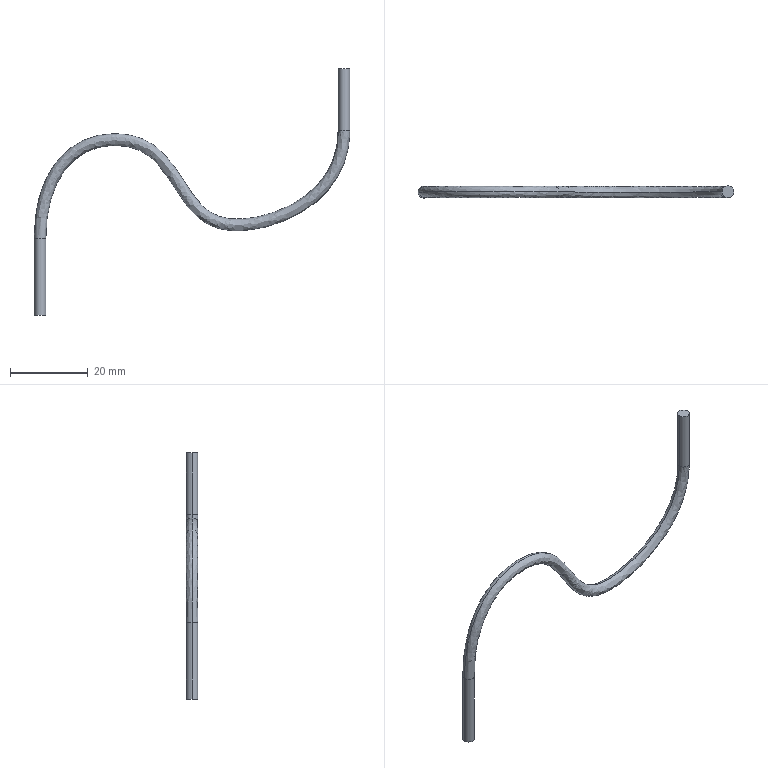Part | SolidWorks | features Sweep 1 | 1 solid | 8 faces | box 81 x 3 x 63.219 mm | volume 1077 mm3 | cylinder 4 | spline 2 | plane 2 | commonest cylinder face diameters 3 x4
STEP:
#1=CARTESIAN_POINT('',(1.5,0.,19.693));
#2=VERTEX_POINT('',#1);
#3=CARTESIAN_POINT('',(-1.5,0.,19.693));
#4=VERTEX_POINT('',#3);
#5=CARTESIAN_POINT('',(0.,0.,19.693));
#6=DIRECTION('',(0.,0.,1.));
#7=DIRECTION('',(1.,0.,0.));
#8=AXIS2_PLACEMENT_3D('',#5,#6,#7);
#9=CIRCLE('',#8,1.5);
#10=EDGE_CURVE('',#2,#4,#9,.T.);
#11=ORIENTED_EDGE('',*,*,#10,.T.);
#12=CARTESIAN_POINT('',(76.5,0.,47.415));
#13=VERTEX_POINT('',#12);
#14=CARTESIAN_POINT('',(-1.5,0.,19.693));
#15=CARTESIAN_POINT('',(-1.5,0.,21.619));
#16=CARTESIAN_POINT('',(-1.286,0.,25.174));
#17=CARTESIAN_POINT('',(-0.3655,0.,30.046));
#18=CARTESIAN_POINT('',(1.116,0.,34.324));
#19=CARTESIAN_POINT('',(3.12,0.,38.02));
#20=CARTESIAN_POINT('',(5.605,0.,41.101));
#21=CARTESIAN_POINT('',(8.521,0.,43.535));
#22=CARTESIAN_POINT('',(11.671,0.,45.218));
#23=CARTESIAN_POINT('',(14.048,0.,45.947));
#24=CARTESIAN_POINT('',(16.493,0.,46.438));
#25=CARTESIAN_POINT('',(19.145,0.,46.678));
#26=CARTESIAN_POINT('',(21.729,0.,46.471));
#27=CARTESIAN_POINT('',(23.985,0.,46.05));
#28=CARTESIAN_POINT('',(26.086,0.,45.432));
#29=CARTESIAN_POINT('',(29.579,0.,43.628));
#30=CARTESIAN_POINT('',(33.041,0.,40.317));
#31=CARTESIAN_POINT('',(36.143,0.,35.723));
#32=CARTESIAN_POINT('',(38.926,0.,31.213));
#33=CARTESIAN_POINT('',(41.349,0.,28.227));
#34=CARTESIAN_POINT('',(43.255,0.,26.716));
#35=CARTESIAN_POINT('',(44.276,0.,26.089));
#36=CARTESIAN_POINT('',(45.357,0.,25.543));
#37=CARTESIAN_POINT('',(46.813,0.,25.02));
#38=CARTESIAN_POINT('',(48.557,0.,24.717));
#39=CARTESIAN_POINT('',(50.199,0.,24.626));
#40=CARTESIAN_POINT('',(52.606,0.,24.658));
#41=CARTESIAN_POINT('',(56.696,0.,25.233));
#42=CARTESIAN_POINT('',(62.394,0.,27.105));
#43=CARTESIAN_POINT('',(67.129,0.,29.763));
#44=CARTESIAN_POINT('',(70.632,0.,32.74));
#45=CARTESIAN_POINT('',(73.067,0.,35.628));
#46=CARTESIAN_POINT('',(74.957,0.,39.));
#47=CARTESIAN_POINT('',(76.193,0.,42.844));
#48=CARTESIAN_POINT('',(76.5,0.,45.884));
#49=CARTESIAN_POINT('',(76.5,0.,47.415));
#50=B_SPLINE_CURVE_WITH_KNOTS('',3,(#14,#15,#16,#17,#18,#19,#20,#21,#22,#23,#24,#25,#26,#27,#28,#29,#30,#31,#32,#33,#34,#35,#36,#37,#38,#39,#40,#41,#42,#43,#44,#45,#46,#47,#48,#49),.UNSPECIFIED.,.F.,.F.,(4,1,1,1,1,1,1,1,1,1,1,1,1,1,1,1,1,1,1,1,1,1,1,1,1,1,1,1,1,1,1,1,1,4),(0.,0.03125,0.0625,0.09375,0.125,0.1562,0.1875,0.2188,0.2463,0.25,0.2812,0.3125,0.317,0.3437,0.375,0.4375,0.5,0.5625,0.625,0.65,0.6638,0.675,0.7,0.725,0.7364,0.75,0.7917,0.8333,0.875,0.9,0.925,0.95,0.975,1.),.UNSPECIFIED.);
#51=EDGE_CURVE('',#4,#13,#50,.T.);
#52=ORIENTED_EDGE('',*,*,#51,.T.);
#53=CARTESIAN_POINT('',(79.5,0.,47.415));
#54=VERTEX_POINT('',#53);
#55=CARTESIAN_POINT('',(78.,0.,47.415));
#56=DIRECTION('',(0.,0.,1.));
#57=DIRECTION('',(1.,0.,0.));
#58=AXIS2_PLACEMENT_3D('',#55,#56,#57);
#59=CIRCLE('',#58,1.5);
#60=EDGE_CURVE('',#54,#13,#59,.T.);
#61=ORIENTED_EDGE('',*,*,#60,.F.);
#62=CARTESIAN_POINT('',(1.5,0.,19.693));
#63=CARTESIAN_POINT('',(1.5,0.,21.529));
#64=CARTESIAN_POINT('',(1.701,0.,24.81));
#65=CARTESIAN_POINT('',(2.548,0.,29.292));
#66=CARTESIAN_POINT('',(3.881,0.,33.125));
#67=CARTESIAN_POINT('',(5.64,0.,36.362));
#68=CARTESIAN_POINT('',(7.767,0.,38.993));
#69=CARTESIAN_POINT('',(10.214,0.,41.032));
#70=CARTESIAN_POINT('',(12.837,0.,42.433));
#71=CARTESIAN_POINT('',(14.816,0.,43.042));
#72=CARTESIAN_POINT('',(16.882,0.,43.456));
#73=CARTESIAN_POINT('',(19.163,0.,43.665));
#74=CARTESIAN_POINT('',(21.382,0.,43.483));
#75=CARTESIAN_POINT('',(23.262,0.,43.134));
#76=CARTESIAN_POINT('',(24.963,0.,42.63));
#77=CARTESIAN_POINT('',(27.763,0.,41.186));
#78=CARTESIAN_POINT('',(30.672,0.,38.439));
#79=CARTESIAN_POINT('',(33.584,0.,34.163));
#80=CARTESIAN_POINT('',(36.417,0.,29.558));
#81=CARTESIAN_POINT('',(39.152,0.,26.143));
#82=CARTESIAN_POINT('',(41.51,0.,24.266));
#83=CARTESIAN_POINT('',(42.806,0.,23.47));
#84=CARTESIAN_POINT('',(44.192,0.,22.769));
#85=CARTESIAN_POINT('',(46.066,0.,22.098));
#86=CARTESIAN_POINT('',(48.215,0.,21.73));
#87=CARTESIAN_POINT('',(50.146,0.,21.624));
#88=CARTESIAN_POINT('',(52.902,0.,21.663));
#89=CARTESIAN_POINT('',(57.393,0.,22.301));
#90=CARTESIAN_POINT('',(63.599,0.,24.338));
#91=CARTESIAN_POINT('',(68.819,0.,27.261));
#92=CARTESIAN_POINT('',(72.76,0.,30.605));
#93=CARTESIAN_POINT('',(75.544,0.,33.901));
#94=CARTESIAN_POINT('',(77.729,0.,37.803));
#95=CARTESIAN_POINT('',(79.155,0.,42.223));
#96=CARTESIAN_POINT('',(79.5,0.,45.734));
#97=CARTESIAN_POINT('',(79.5,0.,47.415));
#98=B_SPLINE_CURVE_WITH_KNOTS('',3,(#62,#63,#64,#65,#66,#67,#68,#69,#70,#71,#72,#73,#74,#75,#76,#77,#78,#79,#80,#81,#82,#83,#84,#85,#86,#87,#88,#89,#90,#91,#92,#93,#94,#95,#96,#97),.UNSPECIFIED.,.F.,.F.,(4,1,1,1,1,1,1,1,1,1,1,1,1,1,1,1,1,1,1,1,1,1,1,1,1,1,1,1,1,1,1,1,1,4),(0.,0.03125,0.0625,0.09375,0.125,0.1562,0.1875,0.2188,0.2463,0.25,0.2812,0.3125,0.317,0.3437,0.375,0.4375,0.5,0.5625,0.625,0.65,0.6638,0.675,0.7,0.725,0.7364,0.75,0.7917,0.8333,0.875,0.9,0.925,0.95,0.975,1.),.UNSPECIFIED.);
#99=EDGE_CURVE('',#2,#54,#98,.T.);
#100=ORIENTED_EDGE('',*,*,#99,.F.);
#101=EDGE_LOOP('',(#11,#52,#61,#100));
#102=FACE_OUTER_BOUND('',#101,.T.);
#103=CARTESIAN_POINT('',(1.5,0.,19.693));
#104=CARTESIAN_POINT('',(1.5,0.,21.529));
#105=CARTESIAN_POINT('',(1.701,0.,24.81));
#106=CARTESIAN_POINT('',(2.548,0.,29.292));
#107=CARTESIAN_POINT('',(3.881,0.,33.125));
#108=CARTESIAN_POINT('',(5.64,0.,36.362));
#109=CARTESIAN_POINT('',(7.767,0.,38.993));
#110=CARTESIAN_POINT('',(10.214,0.,41.032));
#111=CARTESIAN_POINT('',(12.837,0.,42.433));
#112=CARTESIAN_POINT('',(14.816,0.,43.042));
#113=CARTESIAN_POINT('',(16.882,0.,43.456));
#114=CARTESIAN_POINT('',(19.163,0.,43.665));
#115=CARTESIAN_POINT('',(21.382,0.,43.483));
#116=CARTESIAN_POINT('',(23.262,0.,43.134));
#117=CARTESIAN_POINT('',(24.963,0.,42.63));
#118=CARTESIAN_POINT('',(27.763,0.,41.186));
#119=CARTESIAN_POINT('',(30.672,0.,38.439));
#120=CARTESIAN_POINT('',(33.584,0.,34.163));
#121=CARTESIAN_POINT('',(36.417,0.,29.558));
#122=CARTESIAN_POINT('',(39.152,0.,26.143));
#123=CARTESIAN_POINT('',(41.51,0.,24.266));
#124=CARTESIAN_POINT('',(42.806,0.,23.47));
#125=CARTESIAN_POINT('',(44.192,0.,22.769));
#126=CARTESIAN_POINT('',(46.066,0.,22.098));
#127=CARTESIAN_POINT('',(48.215,0.,21.73));
#128=CARTESIAN_POINT('',(50.146,0.,21.624));
#129=CARTESIAN_POINT('',(52.902,0.,21.663));
#130=CARTESIAN_POINT('',(57.393,0.,22.301));
#131=CARTESIAN_POINT('',(63.599,0.,24.338));
#132=CARTESIAN_POINT('',(68.819,0.,27.261));
#133=CARTESIAN_POINT('',(72.76,0.,30.605));
#134=CARTESIAN_POINT('',(75.544,0.,33.901));
#135=CARTESIAN_POINT('',(77.729,0.,37.803));
#136=CARTESIAN_POINT('',(79.155,0.,42.223));
#137=CARTESIAN_POINT('',(79.5,0.,45.734));
#138=CARTESIAN_POINT('',(79.5,0.,47.415));
#139=CARTESIAN_POINT('',(1.5,3.,19.693));
#140=CARTESIAN_POINT('',(1.5,3.,21.709));
#141=CARTESIAN_POINT('',(1.701,3.,24.727));
#142=CARTESIAN_POINT('',(2.548,3.,29.314));
#143=CARTESIAN_POINT('',(3.881,3.,33.119));
#144=CARTESIAN_POINT('',(5.64,3.,36.364));
#145=CARTESIAN_POINT('',(7.767,3.,38.992));
#146=CARTESIAN_POINT('',(10.214,3.,41.032));
#147=CARTESIAN_POINT('',(12.837,3.,42.433));
#148=CARTESIAN_POINT('',(14.816,3.,43.042));
#149=CARTESIAN_POINT('',(16.882,3.,43.456));
#150=CARTESIAN_POINT('',(19.163,3.,43.665));
#151=CARTESIAN_POINT('',(21.382,3.,43.483));
#152=CARTESIAN_POINT('',(23.262,3.,43.134));
#153=CARTESIAN_POINT('',(24.963,3.,42.63));
#154=CARTESIAN_POINT('',(27.763,3.,41.186));
#155=CARTESIAN_POINT('',(30.672,3.,38.439));
#156=CARTESIAN_POINT('',(33.584,3.,34.163));
#157=CARTESIAN_POINT('',(36.417,3.,29.558));
#158=CARTESIAN_POINT('',(39.152,3.,26.143));
#159=CARTESIAN_POINT('',(41.51,3.,24.266));
#160=CARTESIAN_POINT('',(42.806,3.,23.47));
#161=CARTESIAN_POINT('',(44.192,3.,22.769));
#162=CARTESIAN_POINT('',(46.066,3.,22.098));
#163=CARTESIAN_POINT('',(48.215,3.,21.73));
#164=CARTESIAN_POINT('',(50.146,3.,21.624));
#165=CARTESIAN_POINT('',(52.902,3.,21.663));
#166=CARTESIAN_POINT('',(57.393,3.,22.301));
#167=CARTESIAN_POINT('',(63.599,3.,24.338));
#168=CARTESIAN_POINT('',(68.819,3.,27.26));
#169=CARTESIAN_POINT('',(72.76,3.,30.608));
#170=CARTESIAN_POINT('',(75.544,3.,33.891));
#171=CARTESIAN_POINT('',(77.729,3.,37.841));
#172=CARTESIAN_POINT('',(79.155,3.,42.084));
#173=CARTESIAN_POINT('',(79.5,3.,46.035));
#174=CARTESIAN_POINT('',(79.5,3.,47.415));
#175=CARTESIAN_POINT('',(-1.5,3.,19.693));
#176=CARTESIAN_POINT('',(-1.5,3.,21.709));
#177=CARTESIAN_POINT('',(-1.286,3.,25.132));
#178=CARTESIAN_POINT('',(-0.3655,3.,30.057));
#179=CARTESIAN_POINT('',(1.116,3.,34.321));
#180=CARTESIAN_POINT('',(3.12,3.,38.021));
#181=CARTESIAN_POINT('',(5.605,3.,41.101));
#182=CARTESIAN_POINT('',(8.521,3.,43.535));
#183=CARTESIAN_POINT('',(11.671,3.,45.218));
#184=CARTESIAN_POINT('',(14.048,3.,45.947));
#185=CARTESIAN_POINT('',(16.493,3.,46.438));
#186=CARTESIAN_POINT('',(19.145,3.,46.678));
#187=CARTESIAN_POINT('',(21.729,3.,46.471));
#188=CARTESIAN_POINT('',(23.985,3.,46.05));
#189=CARTESIAN_POINT('',(26.086,3.,45.432));
#190=CARTESIAN_POINT('',(29.579,3.,43.628));
#191=CARTESIAN_POINT('',(33.041,3.,40.317));
#192=CARTESIAN_POINT('',(36.143,3.,35.723));
#193=CARTESIAN_POINT('',(38.926,3.,31.213));
#194=CARTESIAN_POINT('',(41.349,3.,28.227));
#195=CARTESIAN_POINT('',(43.255,3.,26.716));
#196=CARTESIAN_POINT('',(44.276,3.,26.089));
#197=CARTESIAN_POINT('',(45.357,3.,25.543));
#198=CARTESIAN_POINT('',(46.813,3.,25.02));
#199=CARTESIAN_POINT('',(48.557,3.,24.717));
#200=CARTESIAN_POINT('',(50.199,3.,24.626));
#201=CARTESIAN_POINT('',(52.606,3.,24.658));
#202=CARTESIAN_POINT('',(56.696,3.,25.233));
#203=CARTESIAN_POINT('',(62.394,3.,27.105));
#204=CARTESIAN_POINT('',(67.129,3.,29.762));
#205=CARTESIAN_POINT('',(70.632,3.,32.741));
#206=CARTESIAN_POINT('',(73.067,3.,35.623));
#207=CARTESIAN_POINT('',(74.957,3.,39.019));
#208=CARTESIAN_POINT('',(76.193,3.,42.775));
#209=CARTESIAN_POINT('',(76.5,3.,46.035));
#210=CARTESIAN_POINT('',(76.5,3.,47.415));
#211=CARTESIAN_POINT('',(-1.5,0.,19.693));
#212=CARTESIAN_POINT('',(-1.5,0.,21.619));
#213=CARTESIAN_POINT('',(-1.286,0.,25.174));
#214=CARTESIAN_POINT('',(-0.3655,0.,30.046));
#215=CARTESIAN_POINT('',(1.116,0.,34.324));
#216=CARTESIAN_POINT('',(3.12,0.,38.02));
#217=CARTESIAN_POINT('',(5.605,0.,41.101));
#218=CARTESIAN_POINT('',(8.521,0.,43.535));
#219=CARTESIAN_POINT('',(11.671,0.,45.218));
#220=CARTESIAN_POINT('',(14.048,0.,45.947));
#221=CARTESIAN_POINT('',(16.493,0.,46.438));
#222=CARTESIAN_POINT('',(19.145,0.,46.678));
#223=CARTESIAN_POINT('',(21.729,0.,46.471));
#224=CARTESIAN_POINT('',(23.985,0.,46.05));
#225=CARTESIAN_POINT('',(26.086,0.,45.432));
#226=CARTESIAN_POINT('',(29.579,0.,43.628));
#227=CARTESIAN_POINT('',(33.041,0.,40.317));
#228=CARTESIAN_POINT('',(36.143,0.,35.723));
#229=CARTESIAN_POINT('',(38.926,0.,31.213));
#230=CARTESIAN_POINT('',(41.349,0.,28.227));
#231=CARTESIAN_POINT('',(43.255,0.,26.716));
#232=CARTESIAN_POINT('',(44.276,0.,26.089));
#233=CARTESIAN_POINT('',(45.357,0.,25.543));
#234=CARTESIAN_POINT('',(46.813,0.,25.02));
#235=CARTESIAN_POINT('',(48.557,0.,24.717));
#236=CARTESIAN_POINT('',(50.199,0.,24.626));
#237=CARTESIAN_POINT('',(52.606,0.,24.658));
#238=CARTESIAN_POINT('',(56.696,0.,25.233));
#239=CARTESIAN_POINT('',(62.394,0.,27.105));
#240=CARTESIAN_POINT('',(67.129,0.,29.763));
#241=CARTESIAN_POINT('',(70.632,0.,32.74));
#242=CARTESIAN_POINT('',(73.067,0.,35.628));
#243=CARTESIAN_POINT('',(74.957,0.,39.));
#244=CARTESIAN_POINT('',(76.193,0.,42.844));
#245=CARTESIAN_POINT('',(76.5,0.,45.884));
#246=CARTESIAN_POINT('',(76.5,0.,47.415));
#247=CARTESIAN_POINT('',(-1.5,-3.,19.693));
#248=CARTESIAN_POINT('',(-1.5,-3.,21.529));
#249=CARTESIAN_POINT('',(-1.286,-3.,25.216));
#250=CARTESIAN_POINT('',(-0.3655,-3.,30.035));
#251=CARTESIAN_POINT('',(1.116,-3.,34.327));
#252=CARTESIAN_POINT('',(3.12,-3.,38.02));
#253=CARTESIAN_POINT('',(5.605,-3.,41.101));
#254=CARTESIAN_POINT('',(8.521,-3.,43.535));
#255=CARTESIAN_POINT('',(11.671,-3.,45.218));
#256=CARTESIAN_POINT('',(14.048,-3.,45.947));
#257=CARTESIAN_POINT('',(16.493,-3.,46.438));
#258=CARTESIAN_POINT('',(19.145,-3.,46.678));
#259=CARTESIAN_POINT('',(21.729,-3.,46.471));
#260=CARTESIAN_POINT('',(23.985,-3.,46.05));
#261=CARTESIAN_POINT('',(26.086,-3.,45.432));
#262=CARTESIAN_POINT('',(29.579,-3.,43.628));
#263=CARTESIAN_POINT('',(33.041,-3.,40.317));
#264=CARTESIAN_POINT('',(36.143,-3.,35.723));
#265=CARTESIAN_POINT('',(38.926,-3.,31.213));
#266=CARTESIAN_POINT('',(41.349,-3.,28.227));
#267=CARTESIAN_POINT('',(43.255,-3.,26.716));
#268=CARTESIAN_POINT('',(44.276,-3.,26.089));
#269=CARTESIAN_POINT('',(45.357,-3.,25.543));
#270=CARTESIAN_POINT('',(46.813,-3.,25.02));
#271=CARTESIAN_POINT('',(48.557,-3.,24.717));
#272=CARTESIAN_POINT('',(50.199,-3.,24.626));
#273=CARTESIAN_POINT('',(52.606,-3.,24.658));
#274=CARTESIAN_POINT('',(56.696,-3.,25.233));
#275=CARTESIAN_POINT('',(62.394,-3.,27.104));
#276=CARTESIAN_POINT('',(67.129,-3.,29.763));
#277=CARTESIAN_POINT('',(70.632,-3.,32.738));
#278=CARTESIAN_POINT('',(73.067,-3.,35.633));
#279=CARTESIAN_POINT('',(74.957,-3.,38.982));
#280=CARTESIAN_POINT('',(76.193,-3.,42.914));
#281=CARTESIAN_POINT('',(76.5,-3.,45.734));
#282=CARTESIAN_POINT('',(76.5,-3.,47.415));
#283=CARTESIAN_POINT('',(1.5,-3.,19.693));
#284=CARTESIAN_POINT('',(1.5,-3.,21.348));
#285=CARTESIAN_POINT('',(1.701,-3.,24.894));
#286=CARTESIAN_POINT('',(2.548,-3.,29.269));
#287=CARTESIAN_POINT('',(3.881,-3.,33.131));
#288=CARTESIAN_POINT('',(5.64,-3.,36.36));
#289=CARTESIAN_POINT('',(7.767,-3.,38.993));
#290=CARTESIAN_POINT('',(10.214,-3.,41.032));
#291=CARTESIAN_POINT('',(12.837,-3.,42.433));
#292=CARTESIAN_POINT('',(14.816,-3.,43.042));
#293=CARTESIAN_POINT('',(16.882,-3.,43.456));
#294=CARTESIAN_POINT('',(19.163,-3.,43.665));
#295=CARTESIAN_POINT('',(21.382,-3.,43.483));
#296=CARTESIAN_POINT('',(23.262,-3.,43.134));
#297=CARTESIAN_POINT('',(24.963,-3.,42.63));
#298=CARTESIAN_POINT('',(27.763,-3.,41.186));
#299=CARTESIAN_POINT('',(30.672,-3.,38.439));
#300=CARTESIAN_POINT('',(33.584,-3.,34.163));
#301=CARTESIAN_POINT('',(36.417,-3.,29.558));
#302=CARTESIAN_POINT('',(39.152,-3.,26.143));
#303=CARTESIAN_POINT('',(41.51,-3.,24.266));
#304=CARTESIAN_POINT('',(42.806,-3.,23.47));
#305=CARTESIAN_POINT('',(44.192,-3.,22.769));
#306=CARTESIAN_POINT('',(46.066,-3.,22.098));
#307=CARTESIAN_POINT('',(48.215,-3.,21.73));
#308=CARTESIAN_POINT('',(50.146,-3.,21.624));
#309=CARTESIAN_POINT('',(52.902,-3.,21.663));
#310=CARTESIAN_POINT('',(57.393,-3.,22.301));
#311=CARTESIAN_POINT('',(63.599,-3.,24.337));
#312=CARTESIAN_POINT('',(68.819,-3.,27.262));
#313=CARTESIAN_POINT('',(72.76,-3.,30.603));
#314=CARTESIAN_POINT('',(75.544,-3.,33.911));
#315=CARTESIAN_POINT('',(77.729,-3.,37.766));
#316=CARTESIAN_POINT('',(79.155,-3.,42.363));
#317=CARTESIAN_POINT('',(79.5,-3.,45.432));
#318=CARTESIAN_POINT('',(79.5,-3.,47.415));
#319=CARTESIAN_POINT('',(1.5,0.,19.693));
#320=CARTESIAN_POINT('',(1.5,0.,21.529));
#321=CARTESIAN_POINT('',(1.701,0.,24.81));
#322=CARTESIAN_POINT('',(2.548,0.,29.292));
#323=CARTESIAN_POINT('',(3.881,0.,33.125));
#324=CARTESIAN_POINT('',(5.64,0.,36.362));
#325=CARTESIAN_POINT('',(7.767,0.,38.993));
#326=CARTESIAN_POINT('',(10.214,0.,41.032));
#327=CARTESIAN_POINT('',(12.837,0.,42.433));
#328=CARTESIAN_POINT('',(14.816,0.,43.042));
#329=CARTESIAN_POINT('',(16.882,0.,43.456));
#330=CARTESIAN_POINT('',(19.163,0.,43.665));
#331=CARTESIAN_POINT('',(21.382,0.,43.483));
#332=CARTESIAN_POINT('',(23.262,0.,43.134));
#333=CARTESIAN_POINT('',(24.963,0.,42.63));
#334=CARTESIAN_POINT('',(27.763,0.,41.186));
#335=CARTESIAN_POINT('',(30.672,0.,38.439));
#336=CARTESIAN_POINT('',(33.584,0.,34.163));
#337=CARTESIAN_POINT('',(36.417,0.,29.558));
#338=CARTESIAN_POINT('',(39.152,0.,26.143));
#339=CARTESIAN_POINT('',(41.51,0.,24.266));
#340=CARTESIAN_POINT('',(42.806,0.,23.47));
#341=CARTESIAN_POINT('',(44.192,0.,22.769));
#342=CARTESIAN_POINT('',(46.066,0.,22.098));
#343=CARTESIAN_POINT('',(48.215,0.,21.73));
#344=CARTESIAN_POINT('',(50.146,0.,21.624));
#345=CARTESIAN_POINT('',(52.902,0.,21.663));
#346=CARTESIAN_POINT('',(57.393,0.,22.301));
#347=CARTESIAN_POINT('',(63.599,0.,24.338));
#348=CARTESIAN_POINT('',(68.819,0.,27.261));
#349=CARTESIAN_POINT('',(72.76,0.,30.605));
#350=CARTESIAN_POINT('',(75.544,0.,33.901));
#351=CARTESIAN_POINT('',(77.729,0.,37.803));
#352=CARTESIAN_POINT('',(79.155,0.,42.223));
#353=CARTESIAN_POINT('',(79.5,0.,45.734));
#354=CARTESIAN_POINT('',(79.5,0.,47.415));
#355=(BOUNDED_SURFACE()B_SPLINE_SURFACE(3,3,((#103,#104,#105,#106,#107,#108,#109,#110,#111,#112,#113,#114,#115,#116,#117,#118,#119,#120,#121,#122,#123,#124,#125,#126,#127,#128,#129,#130,#131,#132,#133,#134,#135,#136,#137,#138),(#139,#140,#141,#142,#143,#144,#145,#146,#147,#148,#149,#150,#151,#152,#153,#154,#155,#156,#157,#158,#159,#160,#161,#162,#163,#164,#165,#166,#167,#168,#169,#170,#171,#172,#173,#174),(#175,#176,#177,#178,#179,#180,#181,#182,#183,#184,#185,#186,#187,#188,#189,#190,#191,#192,#193,#194,#195,#196,#197,#198,#199,#200,#201,#202,#203,#204,#205,#206,#207,#208,#209,#210),(#211,#212,#213,#214,#215,#216,#217,#218,#219,#220,#221,#222,#223,#224,#225,#226,#227,#228,#229,#230,#231,#232,#233,#234,#235,#236,#237,#238,#239,#240,#241,#242,#243,#244,#245,#246),(#247,#248,#249,#250,#251,#252,#253,#254,#255,#256,#257,#258,#259,#260,#261,#262,#263,#264,#265,#266,#267,#268,#269,#270,#271,#272,#273,#274,#275,#276,#277,#278,#279,#280,#281,#282),(#283,#284,#285,#286,#287,#288,#289,#290,#291,#292,#293,#294,#295,#296,#297,#298,#299,#300,#301,#302,#303,#304,#305,#306,#307,#308,#309,#310,#311,#312,#313,#314,#315,#316,#317,#318),(#319,#320,#321,#322,#323,#324,#325,#326,#327,#328,#329,#330,#331,#332,#333,#334,#335,#336,#337,#338,#339,#340,#341,#342,#343,#344,#345,#346,#347,#348,#349,#350,#351,#352,#353,#354)),.UNSPECIFIED.,.T.,.F.,.F.)B_SPLINE_SURFACE_WITH_KNOTS((4,3,4),(4,1,1,1,1,1,1,1,1,1,1,1,1,1,1,1,1,1,1,1,1,1,1,1,1,1,1,1,1,1,1,1,1,4),(0.,0.5,1.),(0.,0.03125,0.0625,0.09375,0.125,0.1562,0.1875,0.2188,0.2463,0.25,0.2812,0.3125,0.317,0.3437,0.375,0.4375,0.5,0.5625,0.625,0.65,0.6638,0.675,0.7,0.725,0.7364,0.75,0.7917,0.8333,0.875,0.9,0.925,0.95,0.975,1.),.UNSPECIFIED.)GEOMETRIC_REPRESENTATION_ITEM()RATIONAL_B_SPLINE_SURFACE(((1.,1.,1.,1.,1.,1.,1.,1.,1.,1.,1.,1.,1.,1.,1.,1.,1.,1.,1.,1.,1.,1.,1.,1.,1.,1.,1.,1.,1.,1.,1.,1.,1.,1.,1.,1.),(0.3333,0.3333,0.3333,0.3333,0.3333,0.3333,0.3333,0.3333,0.3333,0.3333,0.3333,0.3333,0.3333,0.3333,0.3333,0.3333,0.3333,0.3333,0.3333,0.3333,0.3333,0.3333,0.3333,0.3333,0.3333,0.3333,0.3333,0.3333,0.3333,0.3333,0.3333,0.3333,0.3333,0.3333,0.3333,0.3333),(0.3333,0.3333,0.3333,0.3333,0.3333,0.3333,0.3333,0.3333,0.3333,0.3333,0.3333,0.3333,0.3333,0.3333,0.3333,0.3333,0.3333,0.3333,0.3333,0.3333,0.3333,0.3333,0.3333,0.3333,0.3333,0.3333,0.3333,0.3333,0.3333,0.3333,0.3333,0.3333,0.3333,0.3333,0.3333,0.3333),(1.,1.,1.,1.,1.,1.,1.,1.,1.,1.,1.,1.,1.,1.,1.,1.,1.,1.,1.,1.,1.,1.,1.,1.,1.,1.,1.,1.,1.,1.,1.,1.,1.,1.,1.,1.),(0.3333,0.3333,0.3333,0.3333,0.3333,0.3333,0.3333,0.3333,0.3333,0.3333,0.3333,0.3333,0.3333,0.3333,0.3333,0.3333,0.3333,0.3333,0.3333,0.3333,0.3333,0.3333,0.3333,0.3333,0.3333,0.3333,0.3333,0.3333,0.3333,0.3333,0.3333,0.3333,0.3333,0.3333,0.3333,0.3333),(0.3333,0.3333,0.3333,0.3333,0.3333,0.3333,0.3333,0.3333,0.3333,0.3333,0.3333,0.3333,0.3333,0.3333,0.3333,0.3333,0.3333,0.3333,0.3333,0.3333,0.3333,0.3333,0.3333,0.3333,0.3333,0.3333,0.3333,0.3333,0.3333,0.3333,0.3333,0.3333,0.3333,0.3333,0.3333,0.3333),(1.,1.,1.,1.,1.,1.,1.,1.,1.,1.,1.,1.,1.,1.,1.,1.,1.,1.,1.,1.,1.,1.,1.,1.,1.,1.,1.,1.,1.,1.,1.,1.,1.,1.,1.,1.)))REPRESENTATION_ITEM('')SURFACE());
#356=ADVANCED_FACE('',(#102),#355,.T.);
#357=ORIENTED_EDGE('',*,*,#10,.F.);
#358=CARTESIAN_POINT('',(1.5,0.,0.));
#359=VERTEX_POINT('',#358);
#360=CARTESIAN_POINT('',(1.5,0.,19.693));
#361=DIRECTION('',(0.,0.,-1.));
#362=VECTOR('',#361,1000.);
#363=LINE('',#360,#362);
#364=EDGE_CURVE('',#2,#359,#363,.T.);
#365=ORIENTED_EDGE('',*,*,#364,.T.);
#366=CARTESIAN_POINT('',(-1.5,0.,0.));
#367=VERTEX_POINT('',#366);
#368=CARTESIAN_POINT('',(0.,0.,0.));
#369=DIRECTION('',(0.,0.,1.));
#370=DIRECTION('',(1.,0.,0.));
#371=AXIS2_PLACEMENT_3D('',#368,#369,#370);
#372=CIRCLE('',#371,1.5);
#373=EDGE_CURVE('',#359,#367,#372,.T.);
#374=ORIENTED_EDGE('',*,*,#373,.T.);
#375=CARTESIAN_POINT('',(-1.5,0.,19.693));
#376=DIRECTION('',(0.,0.,-1.));
#377=VECTOR('',#376,1000.);
#378=LINE('',#375,#377);
#379=EDGE_CURVE('',#4,#367,#378,.T.);
#380=ORIENTED_EDGE('',*,*,#379,.F.);
#381=EDGE_LOOP('',(#357,#365,#374,#380));
#382=FACE_OUTER_BOUND('',#381,.T.);
#383=CARTESIAN_POINT('',(0.,0.,19.693));
#384=DIRECTION('',(0.,0.,-1.));
#385=DIRECTION('',(-1.,0.,0.));
#386=AXIS2_PLACEMENT_3D('',#383,#384,#385);
#387=CYLINDRICAL_SURFACE('',#386,1.5);
#388=ADVANCED_FACE('',(#382),#387,.T.);
#389=ORIENTED_EDGE('',*,*,#60,.T.);
#390=CARTESIAN_POINT('',(76.5,0.,63.219));
#391=VERTEX_POINT('',#390);
#392=CARTESIAN_POINT('',(76.5,0.,47.415));
#393=DIRECTION('',(0.,0.,1.));
#394=VECTOR('',#393,1000.);
#395=LINE('',#392,#394);
#396=EDGE_CURVE('',#13,#391,#395,.T.);
#397=ORIENTED_EDGE('',*,*,#396,.T.);
#398=CARTESIAN_POINT('',(79.5,0.,63.219));
#399=VERTEX_POINT('',#398);
#400=CARTESIAN_POINT('',(78.,0.,63.219));
#401=DIRECTION('',(0.,0.,1.));
#402=DIRECTION('',(1.,0.,0.));
#403=AXIS2_PLACEMENT_3D('',#400,#401,#402);
#404=CIRCLE('',#403,1.5);
#405=EDGE_CURVE('',#399,#391,#404,.T.);
#406=ORIENTED_EDGE('',*,*,#405,.F.);
#407=CARTESIAN_POINT('',(79.5,0.,47.415));
#408=DIRECTION('',(0.,0.,1.));
#409=VECTOR('',#408,1000.);
#410=LINE('',#407,#409);
#411=EDGE_CURVE('',#54,#399,#410,.T.);
#412=ORIENTED_EDGE('',*,*,#411,.F.);
#413=EDGE_LOOP('',(#389,#397,#406,#412));
#414=FACE_OUTER_BOUND('',#413,.T.);
#415=CARTESIAN_POINT('',(78.,0.,47.415));
#416=DIRECTION('',(0.,0.,1.));
#417=DIRECTION('',(1.,0.,0.));
#418=AXIS2_PLACEMENT_3D('',#415,#416,#417);
#419=CYLINDRICAL_SURFACE('',#418,1.5);
#420=ADVANCED_FACE('',(#414),#419,.T.);
#421=ORIENTED_EDGE('',*,*,#396,.F.);
#422=CARTESIAN_POINT('',(78.,0.,47.415));
#423=DIRECTION('',(0.,0.,1.));
#424=DIRECTION('',(1.,0.,0.));
#425=AXIS2_PLACEMENT_3D('',#422,#423,#424);
#426=CIRCLE('',#425,1.5);
#427=EDGE_CURVE('',#13,#54,#426,.T.);
#428=ORIENTED_EDGE('',*,*,#427,.T.);
#429=ORIENTED_EDGE('',*,*,#411,.T.);
#430=CARTESIAN_POINT('',(78.,0.,63.219));
#431=DIRECTION('',(0.,0.,1.));
#432=DIRECTION('',(1.,0.,0.));
#433=AXIS2_PLACEMENT_3D('',#430,#431,#432);
#434=CIRCLE('',#433,1.5);
#435=EDGE_CURVE('',#391,#399,#434,.T.);
#436=ORIENTED_EDGE('',*,*,#435,.F.);
#437=EDGE_LOOP('',(#421,#428,#429,#436));
#438=FACE_OUTER_BOUND('',#437,.T.);
#439=CARTESIAN_POINT('',(78.,0.,47.415));
#440=DIRECTION('',(0.,0.,1.));
#441=DIRECTION('',(1.,0.,0.));
#442=AXIS2_PLACEMENT_3D('',#439,#440,#441);
#443=CYLINDRICAL_SURFACE('',#442,1.5);
#444=ADVANCED_FACE('',(#438),#443,.T.);
#445=ORIENTED_EDGE('',*,*,#364,.F.);
#446=CARTESIAN_POINT('',(0.,0.,19.693));
#447=DIRECTION('',(0.,0.,1.));
#448=DIRECTION('',(1.,0.,0.));
#449=AXIS2_PLACEMENT_3D('',#446,#447,#448);
#450=CIRCLE('',#449,1.5);
#451=EDGE_CURVE('',#4,#2,#450,.T.);
#452=ORIENTED_EDGE('',*,*,#451,.F.);
#453=ORIENTED_EDGE('',*,*,#379,.T.);
#454=CARTESIAN_POINT('',(0.,0.,0.));
#455=DIRECTION('',(0.,0.,1.));
#456=DIRECTION('',(1.,0.,0.));
#457=AXIS2_PLACEMENT_3D('',#454,#455,#456);
#458=CIRCLE('',#457,1.5);
#459=EDGE_CURVE('',#367,#359,#458,.T.);
#460=ORIENTED_EDGE('',*,*,#459,.T.);
#461=EDGE_LOOP('',(#445,#452,#453,#460));
#462=FACE_OUTER_BOUND('',#461,.T.);
#463=CARTESIAN_POINT('',(0.,0.,19.693));
#464=DIRECTION('',(0.,0.,-1.));
#465=DIRECTION('',(-1.,0.,0.));
#466=AXIS2_PLACEMENT_3D('',#463,#464,#465);
#467=CYLINDRICAL_SURFACE('',#466,1.5);
#468=ADVANCED_FACE('',(#462),#467,.T.);
#469=ORIENTED_EDGE('',*,*,#459,.F.);
#470=ORIENTED_EDGE('',*,*,#373,.F.);
#471=EDGE_LOOP('',(#469,#470));
#472=FACE_OUTER_BOUND('',#471,.T.);
#473=CARTESIAN_POINT('',(0.,0.,0.));
#474=DIRECTION('',(0.,0.,1.));
#475=DIRECTION('',(1.,0.,0.));
#476=AXIS2_PLACEMENT_3D('',#473,#474,#475);
#477=PLANE('',#476);
#478=ADVANCED_FACE('',(#472),#477,.F.);
#479=ORIENTED_EDGE('',*,*,#405,.T.);
#480=ORIENTED_EDGE('',*,*,#435,.T.);
#481=EDGE_LOOP('',(#479,#480));
#482=FACE_OUTER_BOUND('',#481,.T.);
#483=CARTESIAN_POINT('',(78.,0.,63.219));
#484=DIRECTION('',(0.,0.,1.));
#485=DIRECTION('',(1.,0.,0.));
#486=AXIS2_PLACEMENT_3D('',#483,#484,#485);
#487=PLANE('',#486);
#488=ADVANCED_FACE('',(#482),#487,.T.);
#489=ORIENTED_EDGE('',*,*,#51,.F.);
#490=ORIENTED_EDGE('',*,*,#451,.T.);
#491=ORIENTED_EDGE('',*,*,#99,.T.);
#492=ORIENTED_EDGE('',*,*,#427,.F.);
#493=EDGE_LOOP('',(#489,#490,#491,#492));
#494=FACE_OUTER_BOUND('',#493,.T.);
#495=CARTESIAN_POINT('',(1.5,0.,19.693));
#496=CARTESIAN_POINT('',(1.5,0.,21.529));
#497=CARTESIAN_POINT('',(1.701,0.,24.81));
#498=CARTESIAN_POINT('',(2.548,0.,29.292));
#499=CARTESIAN_POINT('',(3.881,0.,33.125));
#500=CARTESIAN_POINT('',(5.64,0.,36.362));
#501=CARTESIAN_POINT('',(7.767,0.,38.993));
#502=CARTESIAN_POINT('',(10.214,0.,41.032));
#503=CARTESIAN_POINT('',(12.837,0.,42.433));
#504=CARTESIAN_POINT('',(14.816,0.,43.042));
#505=CARTESIAN_POINT('',(16.882,0.,43.456));
#506=CARTESIAN_POINT('',(19.163,0.,43.665));
#507=CARTESIAN_POINT('',(21.382,0.,43.483));
#508=CARTESIAN_POINT('',(23.262,0.,43.134));
#509=CARTESIAN_POINT('',(24.963,0.,42.63));
#510=CARTESIAN_POINT('',(27.763,0.,41.186));
#511=CARTESIAN_POINT('',(30.672,0.,38.439));
#512=CARTESIAN_POINT('',(33.584,0.,34.163));
#513=CARTESIAN_POINT('',(36.417,0.,29.558));
#514=CARTESIAN_POINT('',(39.152,0.,26.143));
#515=CARTESIAN_POINT('',(41.51,0.,24.266));
#516=CARTESIAN_POINT('',(42.806,0.,23.47));
#517=CARTESIAN_POINT('',(44.192,0.,22.769));
#518=CARTESIAN_POINT('',(46.066,0.,22.098));
#519=CARTESIAN_POINT('',(48.215,0.,21.73));
#520=CARTESIAN_POINT('',(50.146,0.,21.624));
#521=CARTESIAN_POINT('',(52.902,0.,21.663));
#522=CARTESIAN_POINT('',(57.393,0.,22.301));
#523=CARTESIAN_POINT('',(63.599,0.,24.338));
#524=CARTESIAN_POINT('',(68.819,0.,27.261));
#525=CARTESIAN_POINT('',(72.76,0.,30.605));
#526=CARTESIAN_POINT('',(75.544,0.,33.901));
#527=CARTESIAN_POINT('',(77.729,0.,37.803));
#528=CARTESIAN_POINT('',(79.155,0.,42.223));
#529=CARTESIAN_POINT('',(79.5,0.,45.734));
#530=CARTESIAN_POINT('',(79.5,0.,47.415));
#531=CARTESIAN_POINT('',(1.5,3.,19.693));
#532=CARTESIAN_POINT('',(1.5,3.,21.709));
#533=CARTESIAN_POINT('',(1.701,3.,24.727));
#534=CARTESIAN_POINT('',(2.548,3.,29.314));
#535=CARTESIAN_POINT('',(3.881,3.,33.119));
#536=CARTESIAN_POINT('',(5.64,3.,36.364));
#537=CARTESIAN_POINT('',(7.767,3.,38.992));
#538=CARTESIAN_POINT('',(10.214,3.,41.032));
#539=CARTESIAN_POINT('',(12.837,3.,42.433));
#540=CARTESIAN_POINT('',(14.816,3.,43.042));
#541=CARTESIAN_POINT('',(16.882,3.,43.456));
#542=CARTESIAN_POINT('',(19.163,3.,43.665));
#543=CARTESIAN_POINT('',(21.382,3.,43.483));
#544=CARTESIAN_POINT('',(23.262,3.,43.134));
#545=CARTESIAN_POINT('',(24.963,3.,42.63));
#546=CARTESIAN_POINT('',(27.763,3.,41.186));
#547=CARTESIAN_POINT('',(30.672,3.,38.439));
#548=CARTESIAN_POINT('',(33.584,3.,34.163));
#549=CARTESIAN_POINT('',(36.417,3.,29.558));
#550=CARTESIAN_POINT('',(39.152,3.,26.143));
#551=CARTESIAN_POINT('',(41.51,3.,24.266));
#552=CARTESIAN_POINT('',(42.806,3.,23.47));
#553=CARTESIAN_POINT('',(44.192,3.,22.769));
#554=CARTESIAN_POINT('',(46.066,3.,22.098));
#555=CARTESIAN_POINT('',(48.215,3.,21.73));
#556=CARTESIAN_POINT('',(50.146,3.,21.624));
#557=CARTESIAN_POINT('',(52.902,3.,21.663));
#558=CARTESIAN_POINT('',(57.393,3.,22.301));
#559=CARTESIAN_POINT('',(63.599,3.,24.338));
#560=CARTESIAN_POINT('',(68.819,3.,27.26));
#561=CARTESIAN_POINT('',(72.76,3.,30.608));
#562=CARTESIAN_POINT('',(75.544,3.,33.891));
#563=CARTESIAN_POINT('',(77.729,3.,37.841));
#564=CARTESIAN_POINT('',(79.155,3.,42.084));
#565=CARTESIAN_POINT('',(79.5,3.,46.035));
#566=CARTESIAN_POINT('',(79.5,3.,47.415));
#567=CARTESIAN_POINT('',(-1.5,3.,19.693));
#568=CARTESIAN_POINT('',(-1.5,3.,21.709));
#569=CARTESIAN_POINT('',(-1.286,3.,25.132));
#570=CARTESIAN_POINT('',(-0.3655,3.,30.057));
#571=CARTESIAN_POINT('',(1.116,3.,34.321));
#572=CARTESIAN_POINT('',(3.12,3.,38.021));
#573=CARTESIAN_POINT('',(5.605,3.,41.101));
#574=CARTESIAN_POINT('',(8.521,3.,43.535));
#575=CARTESIAN_POINT('',(11.671,3.,45.218));
#576=CARTESIAN_POINT('',(14.048,3.,45.947));
#577=CARTESIAN_POINT('',(16.493,3.,46.438));
#578=CARTESIAN_POINT('',(19.145,3.,46.678));
#579=CARTESIAN_POINT('',(21.729,3.,46.471));
#580=CARTESIAN_POINT('',(23.985,3.,46.05));
#581=CARTESIAN_POINT('',(26.086,3.,45.432));
#582=CARTESIAN_POINT('',(29.579,3.,43.628));
#583=CARTESIAN_POINT('',(33.041,3.,40.317));
#584=CARTESIAN_POINT('',(36.143,3.,35.723));
#585=CARTESIAN_POINT('',(38.926,3.,31.213));
#586=CARTESIAN_POINT('',(41.349,3.,28.227));
#587=CARTESIAN_POINT('',(43.255,3.,26.716));
#588=CARTESIAN_POINT('',(44.276,3.,26.089));
#589=CARTESIAN_POINT('',(45.357,3.,25.543));
#590=CARTESIAN_POINT('',(46.813,3.,25.02));
#591=CARTESIAN_POINT('',(48.557,3.,24.717));
#592=CARTESIAN_POINT('',(50.199,3.,24.626));
#593=CARTESIAN_POINT('',(52.606,3.,24.658));
#594=CARTESIAN_POINT('',(56.696,3.,25.233));
#595=CARTESIAN_POINT('',(62.394,3.,27.105));
#596=CARTESIAN_POINT('',(67.129,3.,29.762));
#597=CARTESIAN_POINT('',(70.632,3.,32.741));
#598=CARTESIAN_POINT('',(73.067,3.,35.623));
#599=CARTESIAN_POINT('',(74.957,3.,39.019));
#600=CARTESIAN_POINT('',(76.193,3.,42.775));
#601=CARTESIAN_POINT('',(76.5,3.,46.035));
#602=CARTESIAN_POINT('',(76.5,3.,47.415));
#603=CARTESIAN_POINT('',(-1.5,0.,19.693));
#604=CARTESIAN_POINT('',(-1.5,0.,21.619));
#605=CARTESIAN_POINT('',(-1.286,0.,25.174));
#606=CARTESIAN_POINT('',(-0.3655,0.,30.046));
#607=CARTESIAN_POINT('',(1.116,0.,34.324));
#608=CARTESIAN_POINT('',(3.12,0.,38.02));
#609=CARTESIAN_POINT('',(5.605,0.,41.101));
#610=CARTESIAN_POINT('',(8.521,0.,43.535));
#611=CARTESIAN_POINT('',(11.671,0.,45.218));
#612=CARTESIAN_POINT('',(14.048,0.,45.947));
#613=CARTESIAN_POINT('',(16.493,0.,46.438));
#614=CARTESIAN_POINT('',(19.145,0.,46.678));
#615=CARTESIAN_POINT('',(21.729,0.,46.471));
#616=CARTESIAN_POINT('',(23.985,0.,46.05));
#617=CARTESIAN_POINT('',(26.086,0.,45.432));
#618=CARTESIAN_POINT('',(29.579,0.,43.628));
#619=CARTESIAN_POINT('',(33.041,0.,40.317));
#620=CARTESIAN_POINT('',(36.143,0.,35.723));
#621=CARTESIAN_POINT('',(38.926,0.,31.213));
#622=CARTESIAN_POINT('',(41.349,0.,28.227));
#623=CARTESIAN_POINT('',(43.255,0.,26.716));
#624=CARTESIAN_POINT('',(44.276,0.,26.089));
#625=CARTESIAN_POINT('',(45.357,0.,25.543));
#626=CARTESIAN_POINT('',(46.813,0.,25.02));
#627=CARTESIAN_POINT('',(48.557,0.,24.717));
#628=CARTESIAN_POINT('',(50.199,0.,24.626));
#629=CARTESIAN_POINT('',(52.606,0.,24.658));
#630=CARTESIAN_POINT('',(56.696,0.,25.233));
#631=CARTESIAN_POINT('',(62.394,0.,27.105));
#632=CARTESIAN_POINT('',(67.129,0.,29.763));
#633=CARTESIAN_POINT('',(70.632,0.,32.74));
#634=CARTESIAN_POINT('',(73.067,0.,35.628));
#635=CARTESIAN_POINT('',(74.957,0.,39.));
#636=CARTESIAN_POINT('',(76.193,0.,42.844));
#637=CARTESIAN_POINT('',(76.5,0.,45.884));
#638=CARTESIAN_POINT('',(76.5,0.,47.415));
#639=CARTESIAN_POINT('',(-1.5,-3.,19.693));
#640=CARTESIAN_POINT('',(-1.5,-3.,21.529));
#641=CARTESIAN_POINT('',(-1.286,-3.,25.216));
#642=CARTESIAN_POINT('',(-0.3655,-3.,30.035));
#643=CARTESIAN_POINT('',(1.116,-3.,34.327));
#644=CARTESIAN_POINT('',(3.12,-3.,38.02));
#645=CARTESIAN_POINT('',(5.605,-3.,41.101));
#646=CARTESIAN_POINT('',(8.521,-3.,43.535));
#647=CARTESIAN_POINT('',(11.671,-3.,45.218));
#648=CARTESIAN_POINT('',(14.048,-3.,45.947));
#649=CARTESIAN_POINT('',(16.493,-3.,46.438));
#650=CARTESIAN_POINT('',(19.145,-3.,46.678));
#651=CARTESIAN_POINT('',(21.729,-3.,46.471));
#652=CARTESIAN_POINT('',(23.985,-3.,46.05));
#653=CARTESIAN_POINT('',(26.086,-3.,45.432));
#654=CARTESIAN_POINT('',(29.579,-3.,43.628));
#655=CARTESIAN_POINT('',(33.041,-3.,40.317));
#656=CARTESIAN_POINT('',(36.143,-3.,35.723));
#657=CARTESIAN_POINT('',(38.926,-3.,31.213));
#658=CARTESIAN_POINT('',(41.349,-3.,28.227));
#659=CARTESIAN_POINT('',(43.255,-3.,26.716));
#660=CARTESIAN_POINT('',(44.276,-3.,26.089));
#661=CARTESIAN_POINT('',(45.357,-3.,25.543));
#662=CARTESIAN_POINT('',(46.813,-3.,25.02));
#663=CARTESIAN_POINT('',(48.557,-3.,24.717));
#664=CARTESIAN_POINT('',(50.199,-3.,24.626));
#665=CARTESIAN_POINT('',(52.606,-3.,24.658));
#666=CARTESIAN_POINT('',(56.696,-3.,25.233));
#667=CARTESIAN_POINT('',(62.394,-3.,27.104));
#668=CARTESIAN_POINT('',(67.129,-3.,29.763));
#669=CARTESIAN_POINT('',(70.632,-3.,32.738));
#670=CARTESIAN_POINT('',(73.067,-3.,35.633));
#671=CARTESIAN_POINT('',(74.957,-3.,38.982));
#672=CARTESIAN_POINT('',(76.193,-3.,42.914));
#673=CARTESIAN_POINT('',(76.5,-3.,45.734));
#674=CARTESIAN_POINT('',(76.5,-3.,47.415));
#675=CARTESIAN_POINT('',(1.5,-3.,19.693));
#676=CARTESIAN_POINT('',(1.5,-3.,21.348));
#677=CARTESIAN_POINT('',(1.701,-3.,24.894));
#678=CARTESIAN_POINT('',(2.548,-3.,29.269));
#679=CARTESIAN_POINT('',(3.881,-3.,33.131));
#680=CARTESIAN_POINT('',(5.64,-3.,36.36));
#681=CARTESIAN_POINT('',(7.767,-3.,38.993));
#682=CARTESIAN_POINT('',(10.214,-3.,41.032));
#683=CARTESIAN_POINT('',(12.837,-3.,42.433));
#684=CARTESIAN_POINT('',(14.816,-3.,43.042));
#685=CARTESIAN_POINT('',(16.882,-3.,43.456));
#686=CARTESIAN_POINT('',(19.163,-3.,43.665));
#687=CARTESIAN_POINT('',(21.382,-3.,43.483));
#688=CARTESIAN_POINT('',(23.262,-3.,43.134));
#689=CARTESIAN_POINT('',(24.963,-3.,42.63));
#690=CARTESIAN_POINT('',(27.763,-3.,41.186));
#691=CARTESIAN_POINT('',(30.672,-3.,38.439));
#692=CARTESIAN_POINT('',(33.584,-3.,34.163));
#693=CARTESIAN_POINT('',(36.417,-3.,29.558));
#694=CARTESIAN_POINT('',(39.152,-3.,26.143));
#695=CARTESIAN_POINT('',(41.51,-3.,24.266));
#696=CARTESIAN_POINT('',(42.806,-3.,23.47));
#697=CARTESIAN_POINT('',(44.192,-3.,22.769));
#698=CARTESIAN_POINT('',(46.066,-3.,22.098));
#699=CARTESIAN_POINT('',(48.215,-3.,21.73));
#700=CARTESIAN_POINT('',(50.146,-3.,21.624));
#701=CARTESIAN_POINT('',(52.902,-3.,21.663));
#702=CARTESIAN_POINT('',(57.393,-3.,22.301));
#703=CARTESIAN_POINT('',(63.599,-3.,24.337));
#704=CARTESIAN_POINT('',(68.819,-3.,27.262));
#705=CARTESIAN_POINT('',(72.76,-3.,30.603));
#706=CARTESIAN_POINT('',(75.544,-3.,33.911));
#707=CARTESIAN_POINT('',(77.729,-3.,37.766));
#708=CARTESIAN_POINT('',(79.155,-3.,42.363));
#709=CARTESIAN_POINT('',(79.5,-3.,45.432));
#710=CARTESIAN_POINT('',(79.5,-3.,47.415));
#711=CARTESIAN_POINT('',(1.5,0.,19.693));
#712=CARTESIAN_POINT('',(1.5,0.,21.529));
#713=CARTESIAN_POINT('',(1.701,0.,24.81));
#714=CARTESIAN_POINT('',(2.548,0.,29.292));
#715=CARTESIAN_POINT('',(3.881,0.,33.125));
#716=CARTESIAN_POINT('',(5.64,0.,36.362));
#717=CARTESIAN_POINT('',(7.767,0.,38.993));
#718=CARTESIAN_POINT('',(10.214,0.,41.032));
#719=CARTESIAN_POINT('',(12.837,0.,42.433));
#720=CARTESIAN_POINT('',(14.816,0.,43.042));
#721=CARTESIAN_POINT('',(16.882,0.,43.456));
#722=CARTESIAN_POINT('',(19.163,0.,43.665));
#723=CARTESIAN_POINT('',(21.382,0.,43.483));
#724=CARTESIAN_POINT('',(23.262,0.,43.134));
#725=CARTESIAN_POINT('',(24.963,0.,42.63));
#726=CARTESIAN_POINT('',(27.763,0.,41.186));
#727=CARTESIAN_POINT('',(30.672,0.,38.439));
#728=CARTESIAN_POINT('',(33.584,0.,34.163));
#729=CARTESIAN_POINT('',(36.417,0.,29.558));
#730=CARTESIAN_POINT('',(39.152,0.,26.143));
#731=CARTESIAN_POINT('',(41.51,0.,24.266));
#732=CARTESIAN_POINT('',(42.806,0.,23.47));
#733=CARTESIAN_POINT('',(44.192,0.,22.769));
#734=CARTESIAN_POINT('',(46.066,0.,22.098));
#735=CARTESIAN_POINT('',(48.215,0.,21.73));
#736=CARTESIAN_POINT('',(50.146,0.,21.624));
#737=CARTESIAN_POINT('',(52.902,0.,21.663));
#738=CARTESIAN_POINT('',(57.393,0.,22.301));
#739=CARTESIAN_POINT('',(63.599,0.,24.338));
#740=CARTESIAN_POINT('',(68.819,0.,27.261));
#741=CARTESIAN_POINT('',(72.76,0.,30.605));
#742=CARTESIAN_POINT('',(75.544,0.,33.901));
#743=CARTESIAN_POINT('',(77.729,0.,37.803));
#744=CARTESIAN_POINT('',(79.155,0.,42.223));
#745=CARTESIAN_POINT('',(79.5,0.,45.734));
#746=CARTESIAN_POINT('',(79.5,0.,47.415));
#747=(BOUNDED_SURFACE()B_SPLINE_SURFACE(3,3,((#495,#496,#497,#498,#499,#500,#501,#502,#503,#504,#505,#506,#507,#508,#509,#510,#511,#512,#513,#514,#515,#516,#517,#518,#519,#520,#521,#522,#523,#524,#525,#526,#527,#528,#529,#530),(#531,#532,#533,#534,#535,#536,#537,#538,#539,#540,#541,#542,#543,#544,#545,#546,#547,#548,#549,#550,#551,#552,#553,#554,#555,#556,#557,#558,#559,#560,#561,#562,#563,#564,#565,#566),(#567,#568,#569,#570,#571,#572,#573,#574,#575,#576,#577,#578,#579,#580,#581,#582,#583,#584,#585,#586,#587,#588,#589,#590,#591,#592,#593,#594,#595,#596,#597,#598,#599,#600,#601,#602),(#603,#604,#605,#606,#607,#608,#609,#610,#611,#612,#613,#614,#615,#616,#617,#618,#619,#620,#621,#622,#623,#624,#625,#626,#627,#628,#629,#630,#631,#632,#633,#634,#635,#636,#637,#638),(#639,#640,#641,#642,#643,#644,#645,#646,#647,#648,#649,#650,#651,#652,#653,#654,#655,#656,#657,#658,#659,#660,#661,#662,#663,#664,#665,#666,#667,#668,#669,#670,#671,#672,#673,#674),(#675,#676,#677,#678,#679,#680,#681,#682,#683,#684,#685,#686,#687,#688,#689,#690,#691,#692,#693,#694,#695,#696,#697,#698,#699,#700,#701,#702,#703,#704,#705,#706,#707,#708,#709,#710),(#711,#712,#713,#714,#715,#716,#717,#718,#719,#720,#721,#722,#723,#724,#725,#726,#727,#728,#729,#730,#731,#732,#733,#734,#735,#736,#737,#738,#739,#740,#741,#742,#743,#744,#745,#746)),.UNSPECIFIED.,.T.,.F.,.F.)B_SPLINE_SURFACE_WITH_KNOTS((4,3,4),(4,1,1,1,1,1,1,1,1,1,1,1,1,1,1,1,1,1,1,1,1,1,1,1,1,1,1,1,1,1,1,1,1,4),(0.,0.5,1.),(0.,0.03125,0.0625,0.09375,0.125,0.1562,0.1875,0.2188,0.2463,0.25,0.2812,0.3125,0.317,0.3437,0.375,0.4375,0.5,0.5625,0.625,0.65,0.6638,0.675,0.7,0.725,0.7364,0.75,0.7917,0.8333,0.875,0.9,0.925,0.95,0.975,1.),.UNSPECIFIED.)GEOMETRIC_REPRESENTATION_ITEM()RATIONAL_B_SPLINE_SURFACE(((1.,1.,1.,1.,1.,1.,1.,1.,1.,1.,1.,1.,1.,1.,1.,1.,1.,1.,1.,1.,1.,1.,1.,1.,1.,1.,1.,1.,1.,1.,1.,1.,1.,1.,1.,1.),(0.3333,0.3333,0.3333,0.3333,0.3333,0.3333,0.3333,0.3333,0.3333,0.3333,0.3333,0.3333,0.3333,0.3333,0.3333,0.3333,0.3333,0.3333,0.3333,0.3333,0.3333,0.3333,0.3333,0.3333,0.3333,0.3333,0.3333,0.3333,0.3333,0.3333,0.3333,0.3333,0.3333,0.3333,0.3333,0.3333),(0.3333,0.3333,0.3333,0.3333,0.3333,0.3333,0.3333,0.3333,0.3333,0.3333,0.3333,0.3333,0.3333,0.3333,0.3333,0.3333,0.3333,0.3333,0.3333,0.3333,0.3333,0.3333,0.3333,0.3333,0.3333,0.3333,0.3333,0.3333,0.3333,0.3333,0.3333,0.3333,0.3333,0.3333,0.3333,0.3333),(1.,1.,1.,1.,1.,1.,1.,1.,1.,1.,1.,1.,1.,1.,1.,1.,1.,1.,1.,1.,1.,1.,1.,1.,1.,1.,1.,1.,1.,1.,1.,1.,1.,1.,1.,1.),(0.3333,0.3333,0.3333,0.3333,0.3333,0.3333,0.3333,0.3333,0.3333,0.3333,0.3333,0.3333,0.3333,0.3333,0.3333,0.3333,0.3333,0.3333,0.3333,0.3333,0.3333,0.3333,0.3333,0.3333,0.3333,0.3333,0.3333,0.3333,0.3333,0.3333,0.3333,0.3333,0.3333,0.3333,0.3333,0.3333),(0.3333,0.3333,0.3333,0.3333,0.3333,0.3333,0.3333,0.3333,0.3333,0.3333,0.3333,0.3333,0.3333,0.3333,0.3333,0.3333,0.3333,0.3333,0.3333,0.3333,0.3333,0.3333,0.3333,0.3333,0.3333,0.3333,0.3333,0.3333,0.3333,0.3333,0.3333,0.3333,0.3333,0.3333,0.3333,0.3333),(1.,1.,1.,1.,1.,1.,1.,1.,1.,1.,1.,1.,1.,1.,1.,1.,1.,1.,1.,1.,1.,1.,1.,1.,1.,1.,1.,1.,1.,1.,1.,1.,1.,1.,1.,1.)))REPRESENTATION_ITEM('')SURFACE());
#748=ADVANCED_FACE('',(#494),#747,.T.);
#749=CLOSED_SHELL('',(#356,#388,#420,#444,#468,#478,#488,#748));
#750=MANIFOLD_SOLID_BREP('',#749);
#751=CARTESIAN_POINT('',(0.,0.,0.));
#752=DIRECTION('',(0.,0.,1.));
#753=DIRECTION('',(1.,0.,0.));
#754=AXIS2_PLACEMENT_3D('',#751,#752,#753);
#755=(LENGTH_UNIT()NAMED_UNIT(*)SI_UNIT(.MILLI.,.METRE.));
#756=UNCERTAINTY_MEASURE_WITH_UNIT(LENGTH_MEASURE(0.00001),#755,'','');
#757=(NAMED_UNIT(*)PLANE_ANGLE_UNIT()SI_UNIT($,.RADIAN.));
#758=(NAMED_UNIT(*)SI_UNIT($,.STERADIAN.)SOLID_ANGLE_UNIT());
#759=(GEOMETRIC_REPRESENTATION_CONTEXT(3)GLOBAL_UNCERTAINTY_ASSIGNED_CONTEXT((#756))GLOBAL_UNIT_ASSIGNED_CONTEXT((#755,#757,#758))REPRESENTATION_CONTEXT('',''));
#760=ADVANCED_BREP_SHAPE_REPRESENTATION('',(#750,#754),#759);